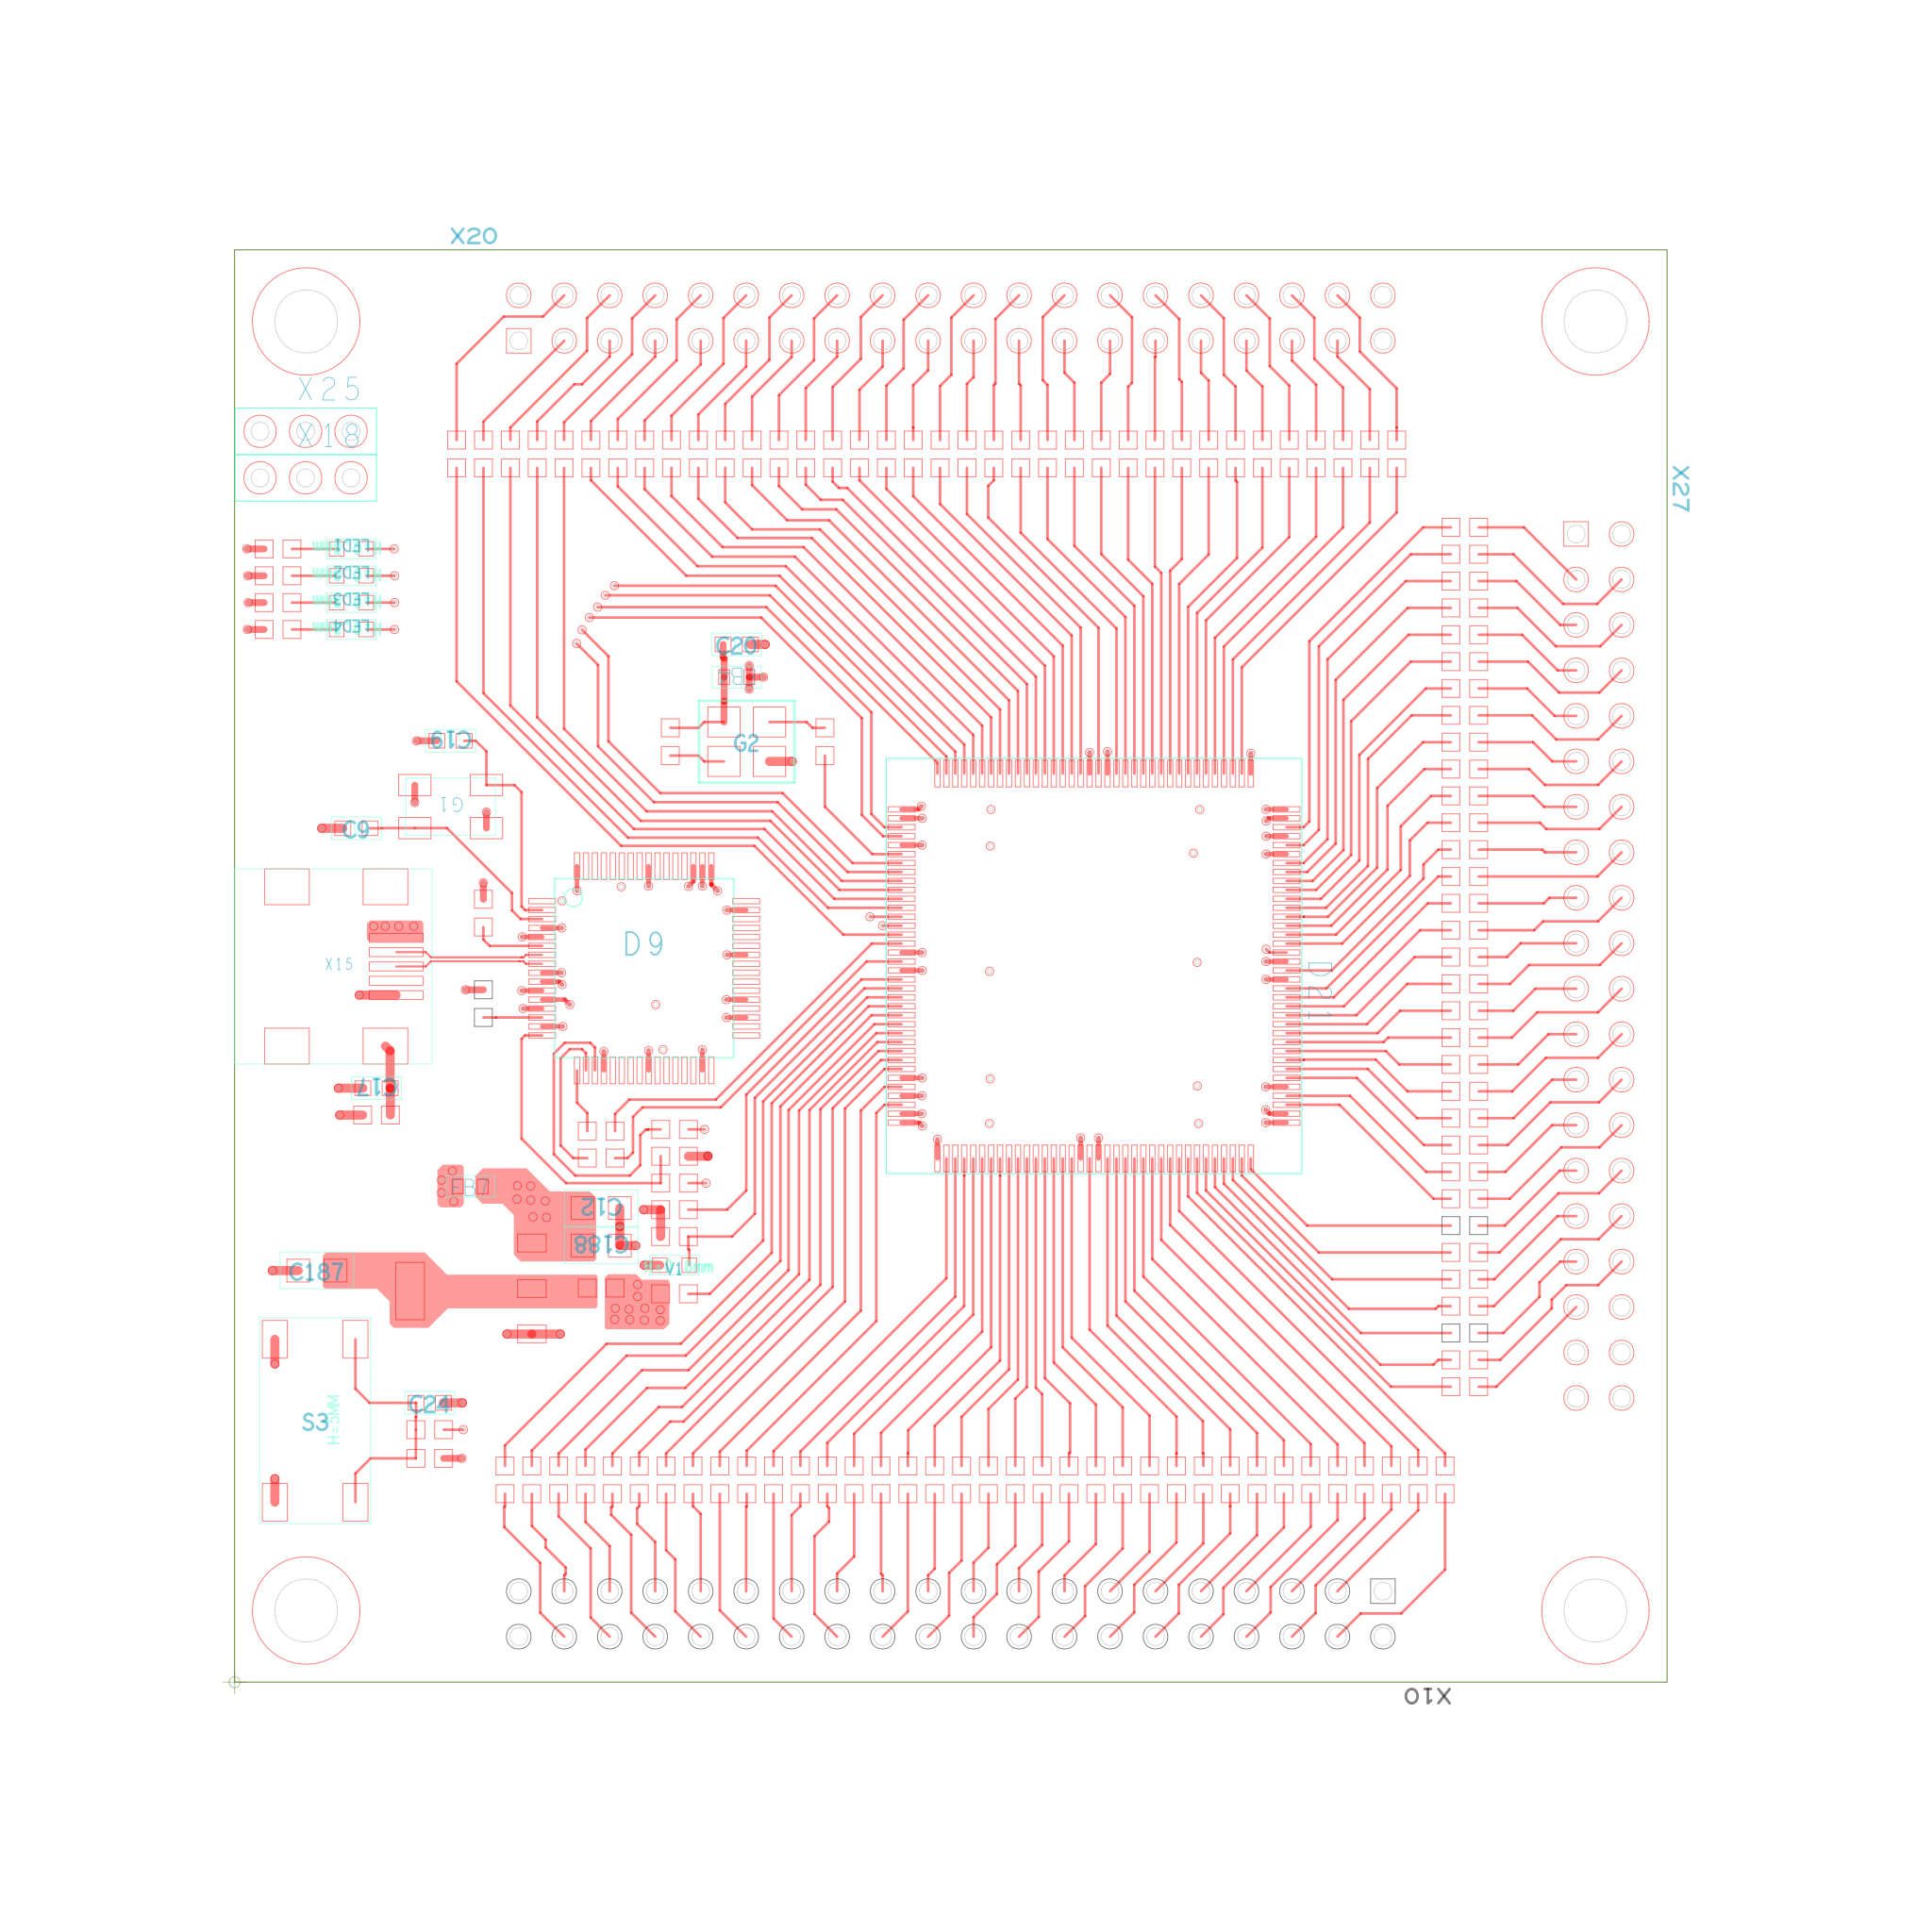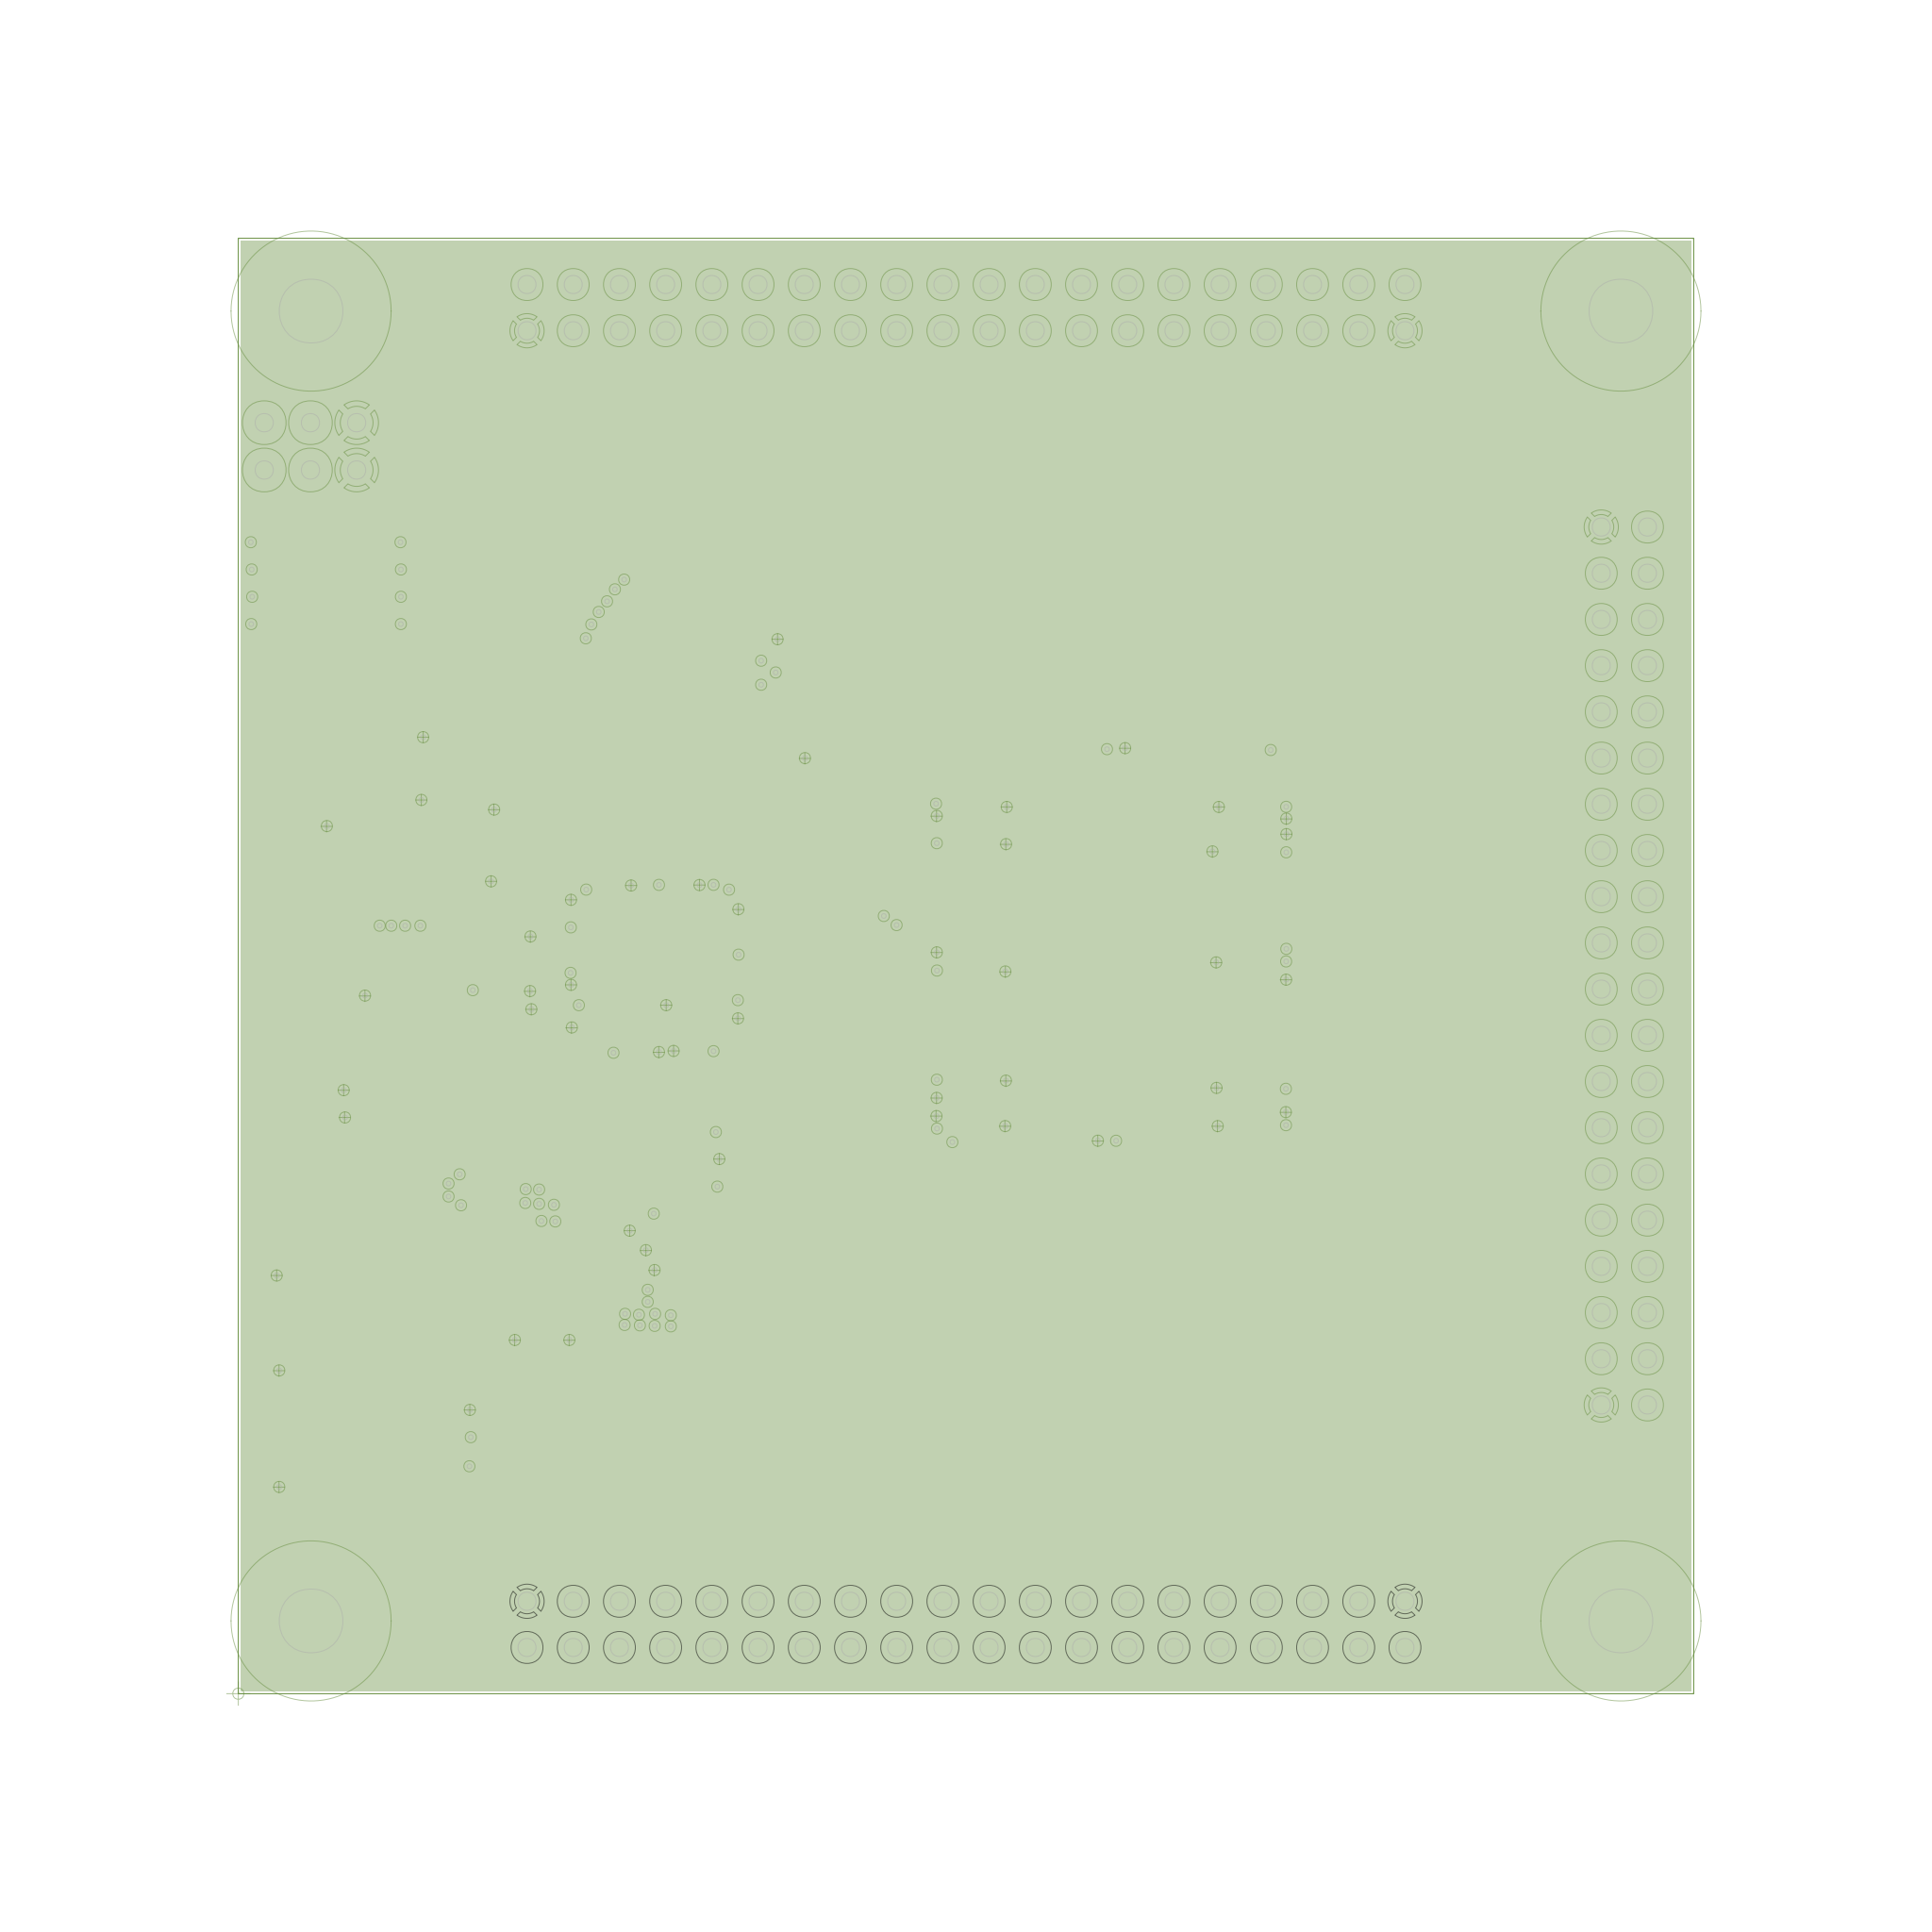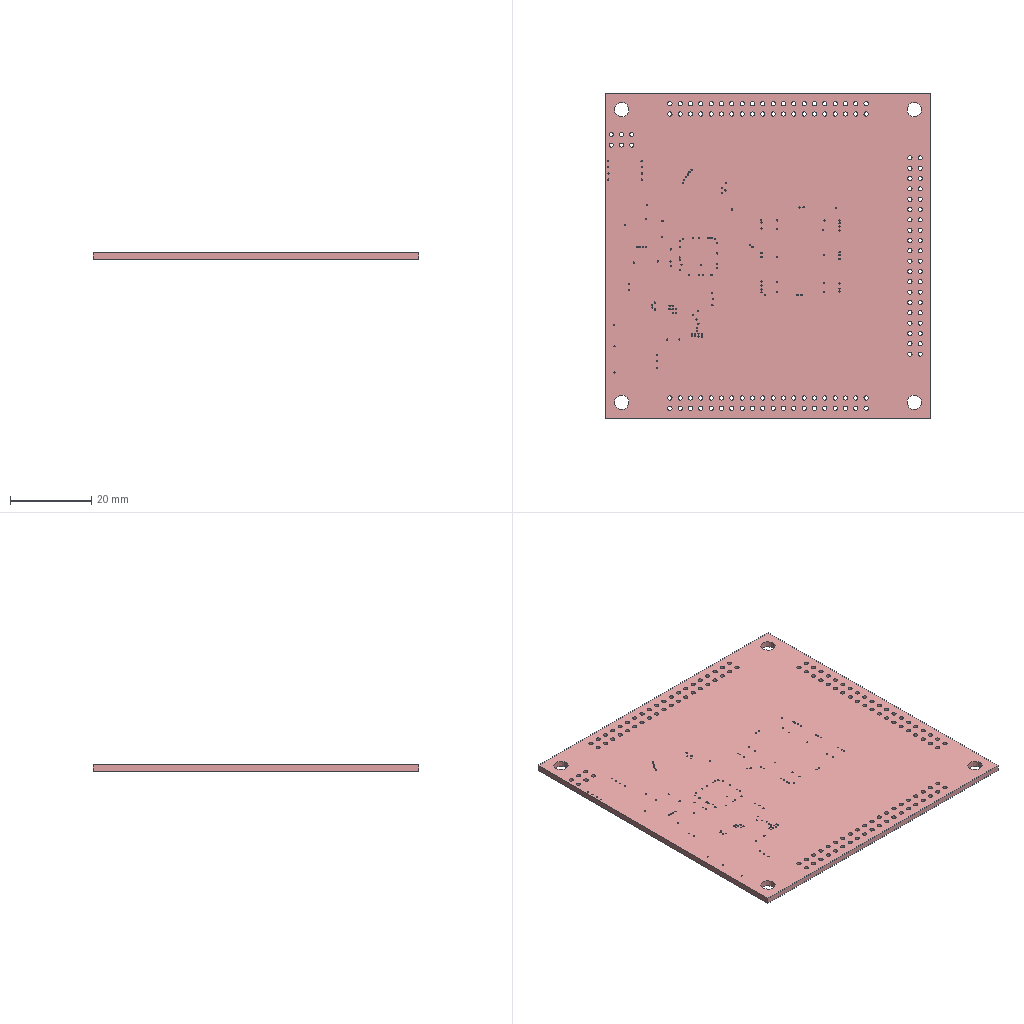Circuit board layout | Cadence Allegro | box 80 x 80 x 1.5 mm
Layer stack:
# Cadence Allegro layer stack of  (unit mm; from the constraint file cross-section; dielectric type: 0 not recorded (Allegro does not mark core vs prepreg), 3 surface material)
index,name,kind,layer,copper_thickness_mm,dielectric_type,dielectric_thickness_mm,dielectric_material,dielectric_constant
0,Top Surface,other,,,,,,
1,TOP,copper,TOP,0.035,,,,
2,Dielectric1,dielectric,,,0,0.1,FR-4,4.5
3,GND,copper,GND,0.0175,,,,
4,Dielectric2,dielectric,,,0,1.265,FR-4,4.5
5,PWR,copper,PWR,0.0175,,,,
6,Dielectric3,dielectric,,,0,0.1,FR-4,4.5
7,BOTTOM,copper,BOTTOM,0.035,,,,
8,Bottom Surface,other,,,,,,
# drill layer pairs: low layer,high layer
drill_pair,TOP,BOTTOM
Part placement:
REFDES,COMP_VALUE,SYM_NAME,SYM_X,SYM_Y,SYM_ROTATE,SYM_MIRROR
C9,22pF,SMC0603,267.961,1877.638,0.000,NO
C11,10nF,SMC0603,1112.000,1471.000,90.000,YES
C12,10uF,C0805,806.024,1042.630,180.000,NO
C13,100nF,SMC0603,881.000,1781.000,0.000,YES
C14,100nF,SMC0603,862.000,1360.000,180.000,YES
C15,100nF,SMC0603,972.000,1360.000,0.000,YES
C16,100nF,SMC0603,690.000,1688.000,270.000,YES
C17,10nF,SMC0603,312.024,1306.087,180.000,NO
C18,100nF,SMC0603,1112.000,1649.000,270.000,YES
C19,22pF,SMC0603,474.960,2070.000,180.000,NO
C20,10nF,SMC0603,1104.000,2282.000,0.000,NO
C22,100nF,SMC0603,690.000,1551.000,90.000,YES
C23,10uF,C0805,836.000,1490.000,0.000,YES
C24,100nF,SMC0603,429.134,614.173,0.000,NO
C187,10uF,C0805,181.000,905.000,0.000,NO
C188,10uF,C0805,806.024,959.953,180.000,NO
C189,100nF,SMC0603,2192.000,1919.000,0.000,YES
C190,100nF,SMC0603,1878.268,1151.417,0.000,YES
C191,100nF,SMC0603,2192.000,1822.835,0.000,YES
C192,100nF,SMC0603,1597.000,1326.772,180.000,YES
C193,100nF,SMC0603,2192.000,2001.063,0.000,YES
C194,100nF,SMC0603,2192.000,1228.346,0.000,YES
C195,100nF,SMC0603,1597.000,1151.417,180.000,YES
C196,100nF,SMC0603,1597.000,1228.346,180.000,YES
C197,100nF,SMC0603,1597.000,1562.992,180.000,YES
C198,100nF,SMC0603,1597.000,1838.583,180.000,YES
C199,100nF,SMC0603,1597.000,1919.000,180.000,YES
C200,100nF,SMC0603,2192.000,1311.024,0.000,YES
C201,100nF,SMC0603,2192.000,1582.677,0.000,YES
C202,100nF,SMC0603,1900.000,2001.063,180.000,YES
D9,FT2232HL,LQFP64_D12_E12_P0R5,900.512,1569.803,0.000,NO
D20,AMS1117-3.3,SOT-223,386.000,860.000,90.000,NO
D21,GW1N-4UV5LQFP144C,QFP144-20X20-P0_5M,1889.764,1574.803,270.000,NO
FB4,MPZ1608S601A,FB0603,1104.000,2210.000,180.000,NO
FB7,MPZ1608S601A NC,FB0603,518.000,1090.000,0.000,NO
G1,25M,RA5032,474.961,1925.307,180.000,NO
G2,25MHZ,OSC4-XO53,1126.000,2068.000,0.000,NO
LED1,LED GREEN,LED0603,256.969,2491.969,180.000,NO
LED2,LED GREEN,LED0603,256.969,2432.913,180.000,NO
LED3,LED GREEN,LED0603,256.969,2373.858,180.000,NO
LED4,LED GREEN,LED0603,256.969,2314.803,180.000,NO
R2,330,R0603,95.551,2314.803,180.000,NO
R8,330,R0603,95.551,2432.913,180.000,NO
R36,330,R0603,95.551,2373.858,180.000,NO
R40,330,R0603,95.551,2491.969,180.000,NO
R175,0,R0603,806.024,1211.535,0.000,NO
R185,12K,R0603,547.000,1691.000,270.000,NO
R191,1K,R0603,967.441,1156.417,180.000,NO
R192,4.7K,R0603,967.173,853.882,180.000,NO
R197,10K,R0603,547.000,1492.000,270.000,NO
R202,22,R0603,1298.000,2068.000,90.000,NO
R203,4.7K,R0603,967.173,1038.921,180.000,NO
R205,4.7K,R0603,967.173,979.866,180.000,NO
R206,33,R0603,429.134,555.118,180.000,NO
R211,0,R0603,806.024,1152.480,0.000,NO
R215,0,R0603,958.000,2068.000,270.000,NO
R218,0,R0603,967.441,1215.472,0.000,NO
R229,0,R0603,967.441,1097.362,0.000,NO
R230,100K,R0603,429.134,492.126,0.000,NO
R232,10K,R0603,312.024,1247.031,180.000,NO
R269,33,R0603,547.244,2700.787,270.000,NO
R270,33,R0603,488.189,2700.787,270.000,NO
R271,33,R0603,665.354,2700.787,270.000,NO
R272,33,R0603,606.299,2700.787,270.000,NO
R273,33,R0603,783.465,2700.787,270.000,NO
R274,33,R0603,724.409,2700.787,270.000,NO
R275,33,R0603,901.575,2700.787,270.000,NO
R276,33,R0603,842.520,2700.787,270.000,NO
R277,33,R0603,1019.685,2700.787,270.000,NO
R278,33,R0603,960.630,2700.787,270.000,NO
R279,33,R0603,1137.795,2700.787,270.000,NO
R280,33,R0603,1078.740,2700.787,270.000,NO
R281,33,R0603,1255.906,2700.787,270.000,NO
R282,33,R0603,1196.850,2700.787,270.000,NO
R283,33,R0603,1374.016,2700.787,270.000,NO
R284,33,R0603,1314.961,2700.787,270.000,NO
R285,33,R0603,1492.126,2700.787,270.000,NO
R286,33,R0603,1433.071,2700.787,270.000,NO
R287,33,R0603,1610.236,2700.787,270.000,NO
R288,33,R0603,1551.181,2700.787,270.000,NO
R289,33,R0603,1728.346,2700.787,270.000,NO
R290,33,R0603,1669.291,2700.787,270.000,NO
R291,33,R0603,1846.457,2700.787,270.000,NO
R292,33,R0603,1787.402,2700.787,270.000,NO
R293,33,R0603,1905.512,2700.787,270.000,NO
R294,33,R0603,1964.567,2700.787,270.000,NO
R295,33,R0603,2023.622,2700.787,270.000,NO
R296,33,R0603,2082.677,2700.787,270.000,NO
R297,33,R0603,2141.732,2700.787,270.000,NO
R298,33,R0603,2200.787,2700.787,270.000,NO
R299,33,R0603,2259.843,2700.787,270.000,NO
R300,33,R0603,2318.898,2700.787,270.000,NO
R301,33,R0603,2377.953,2700.787,270.000,NO
R302,33,R0603,2437.008,2700.787,270.000,NO
R303,33,R0603,2496.063,2700.787,270.000,NO
R304,33,R0603,2555.118,2700.787,270.000,NO
R305,33,R0603,2661.417,444.882,90.000,NO
R306,33,R0603,2484.252,444.882,90.000,NO
R307,33,R0603,2543.307,444.882,90.000,NO
R308,33,R0603,2366.142,444.882,90.000,NO
R309,33,R0603,2425.197,444.882,90.000,NO
R310,33,R0603,2248.031,444.882,90.000,NO
R311,33,R0603,2307.087,444.882,90.000,NO
R312,33,R0603,2129.921,444.882,90.000,NO
R313,33,R0603,2188.976,444.882,90.000,NO
R314,33,R0603,2011.811,444.882,90.000,NO
R315,33,R0603,2070.866,444.882,90.000,NO
R316,33,R0603,1893.701,444.882,90.000,NO
R317,33,R0603,1952.756,444.882,90.000,NO
R318,33,R0603,1775.591,444.882,90.000,NO
R319,33,R0603,1834.646,444.882,90.000,NO
R320,33,R0603,1657.480,444.882,90.000,NO
R321,33,R0603,1716.535,444.882,90.000,NO
R322,33,R0603,1539.370,444.882,90.000,NO
R323,33,R0603,1598.425,444.882,90.000,NO
R324,33,R0603,1421.260,444.882,90.000,NO
R325,33,R0603,1480.315,444.882,90.000,NO
R326,33,R0603,1362.205,444.882,90.000,NO
R327,33,R0603,1303.150,444.882,90.000,NO
R328,33,R0603,1244.094,444.882,90.000,NO
R329,33,R0603,1185.039,444.882,90.000,NO
R330,33,R0603,1125.984,444.882,90.000,NO
R331,33,R0603,1066.929,444.882,90.000,NO
R332,33,R0603,1007.874,444.882,90.000,NO
R333,33,R0603,948.819,444.882,90.000,NO
R334,33,R0603,889.764,444.882,90.000,NO
R335,33,R0603,830.709,444.882,90.000,NO
R336,33,R0603,771.654,444.882,90.000,NO
R337,33,R0603,712.598,444.882,90.000,NO
R338,33,R0603,653.543,444.882,90.000,NO
R339,33,R0603,594.488,444.882,90.000,NO
R340,33,R0603,2602.362,444.882,90.000,NO
R342,0R,R0603,806.024,866.528,180.000,NO
R343,33,R0603,2704.724,708.661,180.000,NO
R344,33,R0603,2704.724,649.606,180.000,NO
R345,33,R0603,2704.724,2539.370,180.000,NO
R346,33,R0603,2704.724,2480.315,180.000,NO
R347,33,R0603,2704.724,2421.260,180.000,NO
R348,33,R0603,2704.724,2362.205,180.000,NO
R349,33,R0603,2704.724,2303.150,180.000,NO
R350,33,R0603,2704.724,2244.094,180.000,NO
R351,33,R0603,2704.724,2185.039,180.000,NO
R352,33,R0603,2704.724,2125.984,180.000,NO
R353,33,R0603,2704.724,2066.929,180.000,NO
R354,33,R0603,2704.724,2007.874,180.000,NO
R355,33,R0603,2704.724,1948.819,180.000,NO
R356,33,R0603,2704.724,1889.764,180.000,NO
R357,33,R0603,2704.724,1830.709,180.000,NO
R358,33,R0603,2704.724,1771.654,180.000,NO
R359,33,R0603,2704.724,1712.598,180.000,NO
R360,33,R0603,2704.724,1653.543,180.000,NO
R361,33,R0603,2704.724,1594.488,180.000,NO
R362,33,R0603,2704.724,1535.433,180.000,NO
R363,33,R0603,2704.724,1476.378,180.000,NO
R364,33,R0603,2704.724,1417.323,180.000,NO
R365,33,R0603,2704.724,1358.268,180.000,NO
R366,33,R0603,2704.724,1299.213,180.000,NO
R367,33,R0603,2704.724,1240.157,180.000,NO
R368,33,R0603,2704.724,1181.102,180.000,NO
R369,33,R0603,2704.724,1122.047,180.000,NO
R370,33,R0603,2704.724,1062.992,180.000,NO
R371,33,R0603,2704.724,1003.937,180.000,NO
R372,33,R0603,2704.724,944.882,180.000,NO
R373,33,R0603,2704.724,885.827,180.000,NO
R374,33,R0603,2704.724,826.772,180.000,NO
R375,33,R0603,2704.724,767.717,180.000,NO
S3,SWITCH,J-SW-4-9_1-E_SWITCH-TL330,177.165,574.803,0.000,NO
V1,LED GREEN,LED0603,967.173,916.874,0.000,NO
X10,40PIN,HEADER2X20-100,2524.803,200.000,180.000,NO
X15,MINI-USB-B,MINIUSBB,355.331,1573.803,0.000,NO
X18,3PIN,SHDR1X3_254-HB11031,56.118,2648.220,0.000,NO
X20,40PIN,HEADER2X20-100,624.803,2949.606,0.000,NO
X25,3PIN,SHDR1X3_254-HB11031,56.118,2750.583,0.000,NO
X27,40PIN,HEADER2X20-100,2949.606,2524.803,270.000,NO
Pad and via stacks:
# Allegro (Cadence) via spans and padstacks; design units: ("mils" 3 1000)
# via spans: padstack,start_layer,end_layer,net_example,count
VIA_10_18,ETCH/TOP,ETCH/BOTTOM,GND,129
# Allegro padstack definitions: name,start_layer,end_layer,drill,plating,holeType,type
SMD_OV36X30,"ETCH/TOP","ETCH/TOP",0.0,"PLATED","none","smd"
SMD_SQ50,"ETCH/TOP","ETCH/TOP",0.0,"PLATED","none","smd"
SMD10X16,"ETCH/TOP","ETCH/TOP",0.0,"PLATED","none","smd"
SMD32X16,"ETCH/TOP","ETCH/TOP",0.0,"PLATED","none","smd"
SMD0_3X1_5,"ETCH/TOP","ETCH/TOP",0.0,"PLATED","none","smd"
R150_30,"ETCH/TOP","ETCH/TOP",0.0,"PLATED","none","smd"
RECT24X32,"ETCH/TOP","ETCH/TOP",0.0,"PLATED","none","smd"
RECT71X47,"ETCH/TOP","ETCH/TOP",0.0,"PLATED","none","smd"
SMD66X71,"ETCH/TOP","ETCH/TOP",0.0,"PLATED","none","smd"
SMD_SQ32,"ETCH/TOP","ETCH/TOP",0.0,"PLATED","none","smd"
SMD39SQU,"ETCH/TOP","ETCH/TOP",0.0,"NON_PLATED","none","smd"
RECT83X55,"ETCH/TOP","ETCH/TOP",0.0,"PLATED","none","smd"
PAD1_8CIR1,"ETCH/TOP","ETCH/BOTTOM",39.402,"PLATED","circle_drill","through"
C054_039,"ETCH/TOP","ETCH/BOTTOM",39.0,"PLATED","circle_drill","through"
S054_039,"ETCH/TOP","ETCH/BOTTOM",39.0,"PLATED","circle_drill","through"
S058_043,"ETCH/TOP","ETCH/BOTTOM",43.0,"PLATED","circle_drill","through"
C058_043,"ETCH/TOP","ETCH/BOTTOM",43.0,"PLATED","circle_drill","through"
RE98_42X78_74,"ETCH/TOP","ETCH/TOP",0.0,"NON_PLATED","none","smd"
RE118_11X19_68,"ETCH/TOP","ETCH/TOP",0.0,"NON_PLATED","none","smd"
RECT35X32,"ETCH/TOP","ETCH/TOP",0.0,"PLATED","none","smd"
VIA,"ETCH/TOP","ETCH/BOTTOM",13.0,"PLATED","circle_drill","through"
TH3P0,"ETCH/TOP","ETCH/BOTTOM",118.11,"PLATED","circle_drill","through"
PLACE-LED3UNIT,"ETCH/TOP","ETCH/BOTTOM",137.799,"PLATED","circle_drill","through"
TH138_CIR118,"ETCH/TOP","ETCH/BOTTOM",137.799,"PLATED","circle_drill","through"
HOLE3P0,"ETCH/TOP","ETCH/BOTTOM",118.11,"PLATED","circle_drill","through"
VIA_10_18,"ETCH/TOP","ETCH/BOTTOM",10.0,"PLATED","circle_drill","through"
Design rules, without the lines most boards share, first 13 of 25 lines:
# Cadence Allegro design rules of  (from the Constraint Manager export constraints.dcfx, design unit mil; typed fields in mm)
# columns: name | kind | enabled | priority | scope1 | scope2 | descriptor | typed fields (field=value)
# Allegro precedence (priority 1 wins): 1 Region class-to-class, 2 Region class, 3 Region, 4 class-to-class, 5 DiffPair/Bus/NetGroup override, 6 NetClass, 7 constraint set (CSet) default
# per-layer values are written LAYER=value in the descriptor and LAYER:mm in the typed field; a maximum of 0 means no limit set
# --- net classes (and buses / net groups) ---
# (no net classes defined: every net uses the default constraint sets)
# --- track widths, neck and differential-pair gap (physical constraint sets) ---
DEFAULT | PhysicalCSet | enabled | 7 | Design default | All | Physical Constraint (Min Line Width=5.78mil) (Max Line Width=0mil) (Min Neck Width=5mil) (Max Neck Length=0mil) (DiffPair Primary Gap=0mil) (DiffPair Neck Gap=0mil) (DiffPair Min Space=0mil) (DiffPair Coupled +Tol=0mil) (DiffPair Coupled -Tol=0mil) (Min BB Via Stagger=5mil) (Max BB Via Stagger=0mil) (T-junctions=ANYWHERE) (Pad-pad direct connect=ALL_ALLOWED) (Allowed vias=VIA_10_18) | min_line_width=0.1468 min_neck_width=0.127 ts_allowed=ANYWHERE min_bvia_stagger=0.127 max_bvia_stagger=0 diffp_primary_gap=0 diffp_neck_gap=0 diffp_coupled_plus=0 diffp_coupled_minus=0 diffp_min_space=0 max_line_width=0 maximum_neck_length=0 allow_on_etch_subclass=TRUE pad_pad_direct_connect=ALL_ALLOWED vias=VIA_10_18
DF90 | PhysicalCSet | enabled | 7 | not referenced | All | Physical Constraint (Min Line Width=4.62mil) (Max Line Width=0mil) (Min Neck Width=4mil) (Max Neck Length=0mil) (DiffPair Primary Gap=4mil) (DiffPair Neck Gap=0mil) (DiffPair Min Space=0mil) (DiffPair Coupled +Tol=0mil) (DiffPair Coupled -Tol=0mil) (Min BB Via Stagger=5mil) (Max BB Via Stagger=0mil) (T-junctions=ANYWHERE) (Pad-pad direct connect=ALL_ALLOWED) (Allowed vias=VIA_10_18) | min_line_width=0.1173 min_neck_width=0.1016 min_bvia_stagger=0.127 max_bvia_stagger=0 ts_allowed=ANYWHERE diffp_primary_gap=0.1016 diffp_neck_gap=0 max_line_width=0 maximum_neck_length=0 pad_pad_direct_connect=ALL_ALLOWED allow_on_etch_subclass=TRUE diffp_coupled_plus=0 diffp_coupled_minus=0 diffp_min_space=0 vias=VIA_10_18
# --- clearances: line / pad / via / shape / hole (spacing constraint sets) ---
DEFAULT | SpacingCSet | enabled | 7 | Design default | All | Clearance Constraint (Line-Line=4mil) (Line-SMD Pad=6mil) (Line-Thru Pin=6mil) (Line-Via=6mil) (Line-Shape=6mil) (SMD Pad-SMD Pad=5mil) (Thru Pin-Thru Pin=5mil) (Thru Pin-SMD Pad=5mil) (SMD Pad-Via=5mil) (Thru Pin-Via=5mil) (Via-Via=5mil) (Shape-SMD Pad=5mil) (Shape-Thru Pin=5mil) (Shape-Via=5mil) (Shape-Shape=5mil) (Hole-Hole=8mil) (Hole-Line=8mil) (Hole-Shape=8mil) (BB Via-BB Via=5mil) (uVia-uVia=5mil) | hole_to_pin_spacing=0.2032 hole_to_via_spacing=0.2032 hole_to_line_spacing=0.2032 hole_to_shape_spacing=0.2032 hole_to_hole_spacing=0.2032 bondpad_to_bondpad_diffp_spc=0.127 mvia_to_mvia_spacing=0.127 mvia_to_thrupin_spacing=0.127 mvia_to_smdpin_spacing=0.127 mvia_to_thruvia_spacing=0.127 mvia_to_bbv_spacing=0.127 mvia_to_line_spacing=0.1524 mvia_to_shape_spacing=0.127 mvia_to_testpin_spacing=0.127 mvia_to_testvia_spacing=0.127 bondpad_to_mvia_spacing=0.127 thrupin_to_thrupin_spacing=0.127 thrupin_to_smdpin_spacing=0.127 thrupin_to_thruvia_spacing=0.127 line_to_thrupin_spacing=0.1524 thrupin_to_shape_spacing=0.127 smdpin_to_smdpin_spacing=0.127 smdpin_to_thruvia_spacing=0.127 line_to_smdpin_spacing=0.1524 shape_to_smdpin_spacing=0.127 thruvia_to_thruvia_spacing=0.127 line_to_thruvia_spacing=0.1524 shape_to_thruvia_spacing=0.127 line_to_line_spacing=0.1016 line_to_shape_spacing=0.1524 shape_to_shape_spacing=0.127 bbv_to_bbv_spacing=0.127 bbv_to_thrupin_spacing=0.127 bbv_to_smdpin_spacing=0.127 bbv_to_thruvia_spacing=0.127 bbv_to_line_spacing=0.1524 bbv_to_shape_spacing=0.127 bbv_to_testpin_spacing=0.127 bbv_to_testvia_spacing=0.127 testpin_to_testpin_spacing=0.127 testpin_to_thrupin_spacing=0.127 smdpin_to_testpin_spacing=0.127 testpin_to_thruvia_spacing=0.127 testpin_to_testvia_spacing=0.127 line_to_testpin_spacing=0.1524 shape_to_testpin_spacing=0.127 testvia_to_testvia_spacing=0.127 testvia_to_thrupin_spacing=0.127 smdpin_to_testvia_spacing=0.127 testvia_to_thruvia_spacing=0.127 line_to_testvia_spacing=0.1524 shape_to_testvia_spacing=0.127 bondpad_to_bondpad_spacing=0.127 thrupin_to_bondpad_spacing=0.127 smdpin_to_bondpad_spacing=0.127 bondpad_to_thruvia_spacing=0.127 bondpad_to_line_spacing=0.1524 bondpad_to_shape_spacing=0.127 bondpad_to_bbv_spacing=0.127 bondpad_to_testpin_spacing=0.127 bondpad_to_testvia_spacing=0.127 min_bvia_gap=0.127
DEFAULT | SameNetSpacingCSet | enabled | 7 | Design default | All | Same-Net Clearance (Line-Line=5mil) (Line-SMD Pad=5mil) (Line-Thru Pin=5mil) (Line-Via=5mil) (Line-Shape=5mil) (SMD Pad-SMD Pad=5mil) (Thru Pin-Thru Pin=5mil) (Thru Pin-SMD Pad=5mil) (SMD Pad-Via=5mil) (Thru Pin-Via=5mil) (Via-Via=5mil) (Shape-SMD Pad=5mil) (Shape-Thru Pin=5mil) (Shape-Via=5mil) (Shape-Shape=5mil) (Hole-Hole=8mil) (Hole-Line=8mil) (Hole-Shape=8mil) (BB Via-BB Via=5mil) (uVia-uVia=5mil) | sn_thrupin_to_thrupin_spacing=0.127 sn_thrupin_to_smdpin_spacing=0.127 sn_thrupin_to_thruvia_spacing=0.127 sn_line_to_thrupin_spacing=0.127 sn_thrupin_to_shape_spacing=0.127 sn_smdpin_to_smdpin_spacing=0.127 sn_smdpin_to_thruvia_spacing=0.127 sn_line_to_smdpin_spacing=0.127 sn_shape_to_smdpin_spacing=0.127 sn_thruvia_to_thruvia_spacing=0.127 sn_line_to_thruvia_spacing=0.127 sn_shape_to_thruvia_spacing=0.127 sn_line_to_line_spacing=0.127 sn_line_to_shape_spacing=0.127 sn_shape_to_shape_spacing=0.127 sn_bbv_to_bbv_spacing=0.127 sn_bbv_to_thrupin_spacing=0.127 sn_bbv_to_smdpin_spacing=0.127 sn_bbv_to_thruvia_spacing=0.127 sn_bbv_to_line_spacing=0.127 sn_bbv_to_shape_spacing=0.127 sn_bbv_to_testpin_spacing=0.127 sn_bbv_to_testvia_spacing=0.127 sn_testpin_to_testpin_spacing=0.127 sn_testpin_to_thrupin_spacing=0.127 sn_smdpin_to_testpin_spacing=0.127 sn_testpin_to_thruvia_spacing=0.127 sn_testpin_to_testvia_spacing=0.127 sn_line_to_testpin_spacing=0.127 sn_shape_to_testpin_spacing=0.127 sn_testvia_to_testvia_spacing=0.127 sn_testvia_to_thrupin_spacing=0.127 sn_smdpin_to_testvia_spacing=0.127 sn_testvia_to_thruvia_spacing=0.127 sn_line_to_testvia_spacing=0.127 sn_shape_to_testvia_spacing=0.127 sn_bondpad_to_bondpad_spacing=0.127 sn_thrupin_to_bondpad_spacing=0.127 sn_smdpin_to_bondpad_spacing=0.127 sn_bondpad_to_thruvia_spacing=0.127 sn_bondpad_to_line_spacing=0.127 sn_bondpad_to_shape_spacing=0.127 sn_bondpad_to_bbv_spacing=0.127 sn_bondpad_to_testpin_spacing=0.127 sn_bondpad_to_testvia_spacing=0.127 same_net=TRUE sn_hole_to_pin_spacing=0.2032 sn_hole_to_via_spacing=0.2032 sn_hole_to_line_spacing=0.2032 sn_hole_to_shape_spacing=0.2032 sn_hole_to_hole_spacing=0.2032 sn_mvia_to_mvia_spacing=0.127 sn_mvia_to_thrupin_spacing=0.127 sn_mvia_to_smdpin_spacing=0.127 sn_mvia_to_thruvia_spacing=0.127 sn_mvia_to_bbv_spacing=0.127 sn_mvia_to_line_spacing=0.127 sn_mvia_to_shape_spacing=0.127 sn_mvia_to_testpin_spacing=0.127 sn_mvia_to_testvia_spacing=0.127 sn_bondpad_to_mvia_spacing=0.127
# --- differential pairs (1) ---